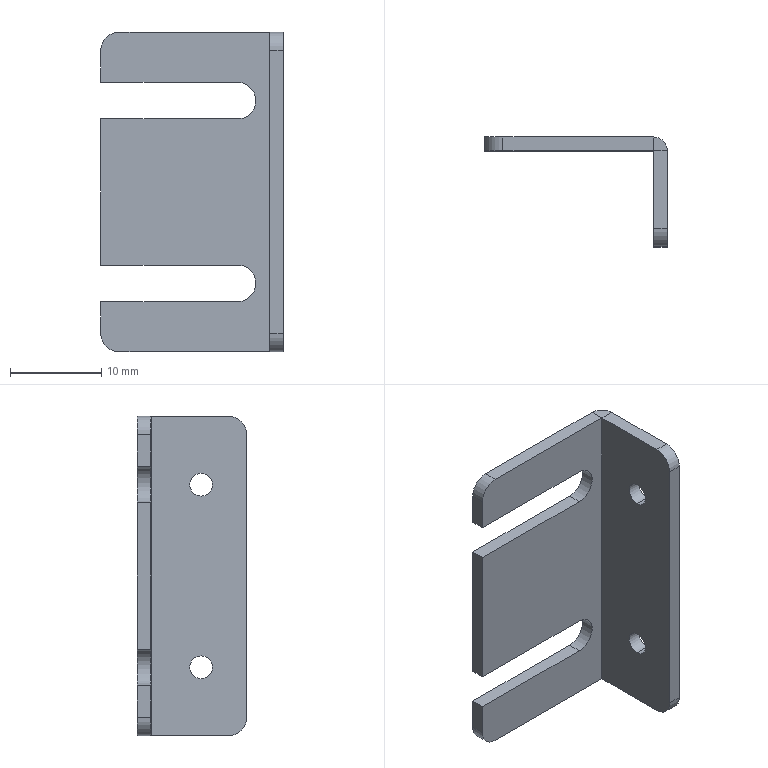Part | STEP file | magnet mounting plate | 1 solid | 30 faces | box 20 x 12 x 35 mm | volume 1365 mm3 | plane 18 | cylinder 12 | commonest cylinder face diameters 4 x6 2.5 x4 0.02 x1 3.02 x1